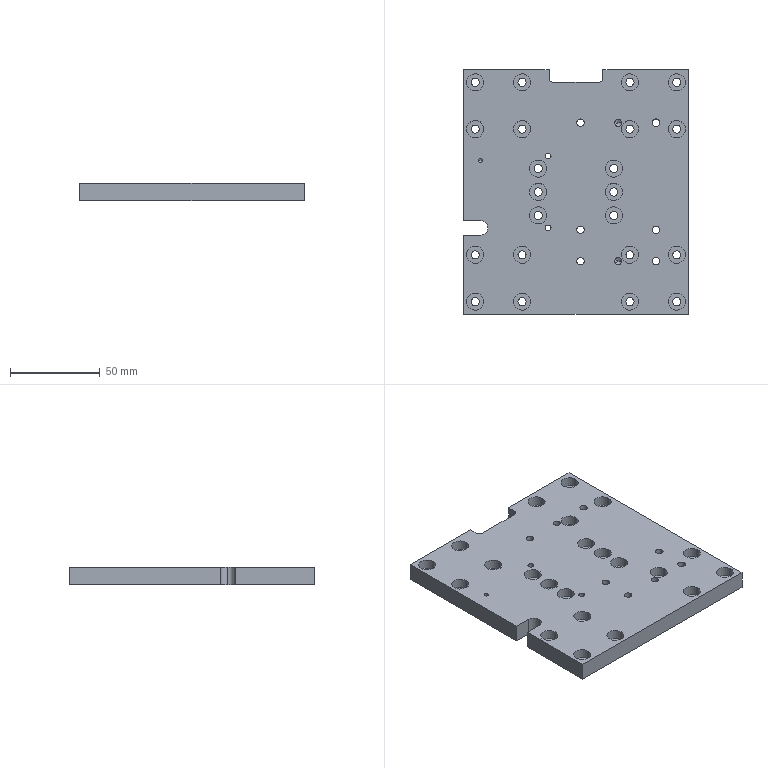Part | STEP file | 1 solid | 195 faces | box 125 x 136 x 10 mm | volume 154591 mm3 | cylinder 134 | plane 35 | cone 26 | commonest cylinder face diameters 4.5 x44 9.5 x44 3.3 x12 4 x12 4.2 x12 2.5 x6